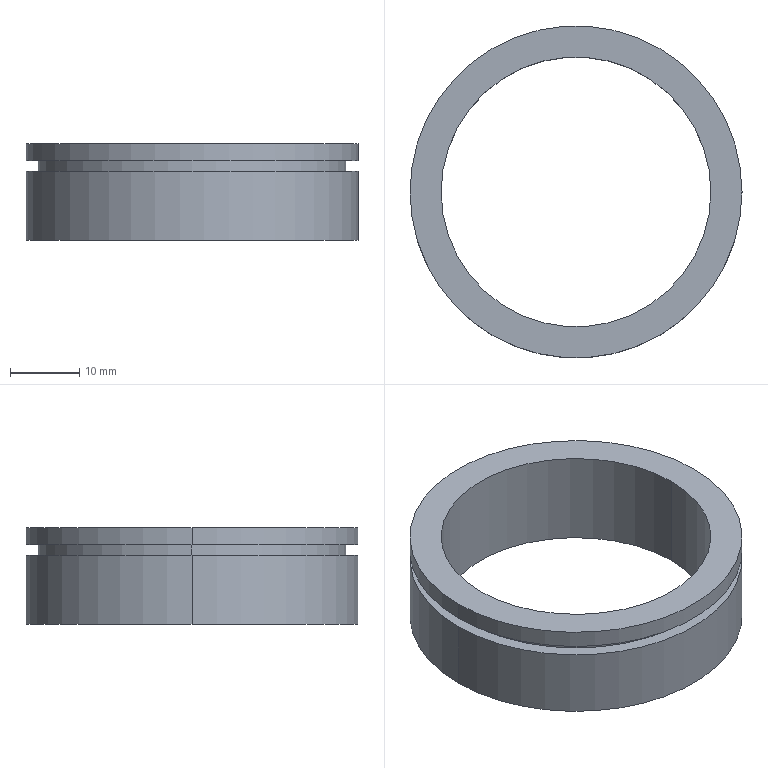Part | STEP file | Nylon bushing QY-1-28 | 1 solid | 12 faces | box 48 x 48 x 14 mm | volume 8228 mm3 | cylinder 8 | plane 4 | commonest cylinder face diameters 48 x4 39 x2 44.5 x2
STEP:
#1=CARTESIAN_POINT('',(0.,0.,0.));
#2=DIRECTION('',(0.,0.,1.));
#3=DIRECTION('',(1.,0.,0.));
#4=AXIS2_PLACEMENT_3D('',#1,#2,#3);
#5=CARTESIAN_POINT('',(22.25,0.,10.));
#6=VERTEX_POINT('',#5);
#7=CARTESIAN_POINT('',(-22.25,0.,10.));
#8=VERTEX_POINT('',#7);
#9=CARTESIAN_POINT('',(0.,0.,10.));
#10=DIRECTION('',(0.,0.,1.));
#11=DIRECTION('',(1.,0.,0.));
#12=AXIS2_PLACEMENT_3D('',#9,#10,#11);
#13=CIRCLE('',#12,22.25);
#14=CARTESIAN_POINT('',(0.,0.,10.));
#15=DIRECTION('',(0.,0.,1.));
#16=DIRECTION('',(1.,0.,0.));
#17=AXIS2_PLACEMENT_3D('',#14,#15,#16);
#18=CYLINDRICAL_SURFACE('',#17,22.25);
#19=CARTESIAN_POINT('',(0.,0.));
#20=DIRECTION('',(1.,0.));
#21=VECTOR('',#20,1.);
#22=LINE('',#19,#21);
#23=(GEOMETRIC_REPRESENTATION_CONTEXT(2)PARAMETRIC_REPRESENTATION_CONTEXT()REPRESENTATION_CONTEXT('',''));
#24=DEFINITIONAL_REPRESENTATION('',(#22),#23);
#25=PCURVE('',#18,#24);
#26=CARTESIAN_POINT('',(0.,0.,10.));
#27=DIRECTION('',(0.,0.,1.));
#28=DIRECTION('',(1.,0.,0.));
#29=AXIS2_PLACEMENT_3D('',#26,#27,#28);
#30=PLANE('',#29);
#31=CARTESIAN_POINT('',(0.,0.));
#32=DIRECTION('',(1.,0.));
#33=AXIS2_PLACEMENT_2D('',#31,#32);
#34=CIRCLE('',#33,22.25);
#35=(GEOMETRIC_REPRESENTATION_CONTEXT(2)PARAMETRIC_REPRESENTATION_CONTEXT()REPRESENTATION_CONTEXT('',''));
#36=DEFINITIONAL_REPRESENTATION('',(#34),#35);
#37=PCURVE('',#30,#36);
#38=SURFACE_CURVE('',#13,(#25,#37),.PCURVE_S1.);
#39=EDGE_CURVE('',#6,#8,#38,.T.);
#40=ORIENTED_EDGE('',*,*,#39,.T.);
#41=CARTESIAN_POINT('',(-22.25,0.,11.5));
#42=VERTEX_POINT('',#41);
#43=CARTESIAN_POINT('',(-22.25,0.,10.));
#44=DIRECTION('',(0.,0.,1.));
#45=VECTOR('',#44,1.);
#46=LINE('',#43,#45);
#47=CARTESIAN_POINT('',(3.142,0.));
#48=DIRECTION('',(0.,1.));
#49=VECTOR('',#48,1.);
#50=LINE('',#47,#49);
#51=(GEOMETRIC_REPRESENTATION_CONTEXT(2)PARAMETRIC_REPRESENTATION_CONTEXT()REPRESENTATION_CONTEXT('',''));
#52=DEFINITIONAL_REPRESENTATION('',(#50),#51);
#53=PCURVE('',#18,#52);
#54=CARTESIAN_POINT('',(0.,0.,10.));
#55=DIRECTION('',(0.,0.,1.));
#56=DIRECTION('',(1.,0.,0.));
#57=AXIS2_PLACEMENT_3D('',#54,#55,#56);
#58=CYLINDRICAL_SURFACE('',#57,22.25);
#59=CARTESIAN_POINT('',(3.142,0.));
#60=DIRECTION('',(0.,1.));
#61=VECTOR('',#60,1.);
#62=LINE('',#59,#61);
#63=(GEOMETRIC_REPRESENTATION_CONTEXT(2)PARAMETRIC_REPRESENTATION_CONTEXT()REPRESENTATION_CONTEXT('',''));
#64=DEFINITIONAL_REPRESENTATION('',(#62),#63);
#65=PCURVE('',#58,#64);
#66=SURFACE_CURVE('',#46,(#53,#65),.PCURVE_S1.);
#67=EDGE_CURVE('',#8,#42,#66,.T.);
#68=ORIENTED_EDGE('',*,*,#67,.T.);
#69=CARTESIAN_POINT('',(22.25,0.,11.5));
#70=VERTEX_POINT('',#69);
#71=CARTESIAN_POINT('',(0.,0.,11.5));
#72=DIRECTION('',(0.,0.,1.));
#73=DIRECTION('',(1.,0.,0.));
#74=AXIS2_PLACEMENT_3D('',#71,#72,#73);
#75=CIRCLE('',#74,22.25);
#76=CARTESIAN_POINT('',(0.,1.5));
#77=DIRECTION('',(1.,0.));
#78=VECTOR('',#77,1.);
#79=LINE('',#76,#78);
#80=(GEOMETRIC_REPRESENTATION_CONTEXT(2)PARAMETRIC_REPRESENTATION_CONTEXT()REPRESENTATION_CONTEXT('',''));
#81=DEFINITIONAL_REPRESENTATION('',(#79),#80);
#82=PCURVE('',#18,#81);
#83=CARTESIAN_POINT('',(0.,0.,11.5));
#84=DIRECTION('',(0.,0.,1.));
#85=DIRECTION('',(1.,0.,0.));
#86=AXIS2_PLACEMENT_3D('',#83,#84,#85);
#87=PLANE('',#86);
#88=CARTESIAN_POINT('',(0.,0.));
#89=DIRECTION('',(1.,0.));
#90=AXIS2_PLACEMENT_2D('',#88,#89);
#91=CIRCLE('',#90,22.25);
#92=(GEOMETRIC_REPRESENTATION_CONTEXT(2)PARAMETRIC_REPRESENTATION_CONTEXT()REPRESENTATION_CONTEXT('',''));
#93=DEFINITIONAL_REPRESENTATION('',(#91),#92);
#94=PCURVE('',#87,#93);
#95=SURFACE_CURVE('',#75,(#82,#94),.PCURVE_S1.);
#96=EDGE_CURVE('',#70,#42,#95,.T.);
#97=ORIENTED_EDGE('',*,*,#96,.F.);
#98=CARTESIAN_POINT('',(22.25,0.,10.));
#99=DIRECTION('',(0.,0.,1.));
#100=VECTOR('',#99,1.);
#101=LINE('',#98,#100);
#102=CARTESIAN_POINT('',(0.,0.));
#103=DIRECTION('',(0.,1.));
#104=VECTOR('',#103,1.);
#105=LINE('',#102,#104);
#106=(GEOMETRIC_REPRESENTATION_CONTEXT(2)PARAMETRIC_REPRESENTATION_CONTEXT()REPRESENTATION_CONTEXT('',''));
#107=DEFINITIONAL_REPRESENTATION('',(#105),#106);
#108=PCURVE('',#18,#107);
#109=CARTESIAN_POINT('',(6.283,0.));
#110=DIRECTION('',(0.,1.));
#111=VECTOR('',#110,1.);
#112=LINE('',#109,#111);
#113=(GEOMETRIC_REPRESENTATION_CONTEXT(2)PARAMETRIC_REPRESENTATION_CONTEXT()REPRESENTATION_CONTEXT('',''));
#114=DEFINITIONAL_REPRESENTATION('',(#112),#113);
#115=PCURVE('',#58,#114);
#116=SURFACE_CURVE('',#101,(#108,#115),.PCURVE_S1.);
#117=EDGE_CURVE('',#6,#70,#116,.T.);
#118=ORIENTED_EDGE('',*,*,#117,.F.);
#119=EDGE_LOOP('',(#40,#68,#97,#118));
#120=FACE_BOUND('',#119,.T.);
#121=ADVANCED_FACE('',(#120),#18,.T.);
#122=CARTESIAN_POINT('',(-19.5,0.,14.));
#123=VERTEX_POINT('',#122);
#124=CARTESIAN_POINT('',(-19.5,0.,0.));
#125=VERTEX_POINT('',#124);
#126=CARTESIAN_POINT('',(-19.5,0.,14.));
#127=DIRECTION('',(0.,0.,-1.));
#128=VECTOR('',#127,1.);
#129=LINE('',#126,#128);
#130=CARTESIAN_POINT('',(0.,0.,14.));
#131=DIRECTION('',(0.,0.,-1.));
#132=DIRECTION('',(-1.,0.,0.));
#133=AXIS2_PLACEMENT_3D('',#130,#131,#132);
#134=CYLINDRICAL_SURFACE('',#133,19.5);
#135=CARTESIAN_POINT('',(6.283,0.));
#136=DIRECTION('',(0.,1.));
#137=VECTOR('',#136,1.);
#138=LINE('',#135,#137);
#139=(GEOMETRIC_REPRESENTATION_CONTEXT(2)PARAMETRIC_REPRESENTATION_CONTEXT()REPRESENTATION_CONTEXT('',''));
#140=DEFINITIONAL_REPRESENTATION('',(#138),#139);
#141=PCURVE('',#134,#140);
#142=CARTESIAN_POINT('',(0.,0.,14.));
#143=DIRECTION('',(0.,0.,-1.));
#144=DIRECTION('',(-1.,0.,0.));
#145=AXIS2_PLACEMENT_3D('',#142,#143,#144);
#146=CYLINDRICAL_SURFACE('',#145,19.5);
#147=CARTESIAN_POINT('',(0.,0.));
#148=DIRECTION('',(0.,1.));
#149=VECTOR('',#148,1.);
#150=LINE('',#147,#149);
#151=(GEOMETRIC_REPRESENTATION_CONTEXT(2)PARAMETRIC_REPRESENTATION_CONTEXT()REPRESENTATION_CONTEXT('',''));
#152=DEFINITIONAL_REPRESENTATION('',(#150),#151);
#153=PCURVE('',#146,#152);
#154=SURFACE_CURVE('',#129,(#141,#153),.PCURVE_S1.);
#155=EDGE_CURVE('',#123,#125,#154,.T.);
#156=ORIENTED_EDGE('',*,*,#155,.T.);
#157=CARTESIAN_POINT('',(19.5,0.,0.));
#158=VERTEX_POINT('',#157);
#159=CARTESIAN_POINT('',(0.,0.,0.));
#160=DIRECTION('',(0.,0.,1.));
#161=DIRECTION('',(1.,0.,0.));
#162=AXIS2_PLACEMENT_3D('',#159,#160,#161);
#163=CIRCLE('',#162,19.5);
#164=CARTESIAN_POINT('',(9.425,14.));
#165=DIRECTION('',(-1.,0.));
#166=VECTOR('',#165,1.);
#167=LINE('',#164,#166);
#168=(GEOMETRIC_REPRESENTATION_CONTEXT(2)PARAMETRIC_REPRESENTATION_CONTEXT()REPRESENTATION_CONTEXT('',''));
#169=DEFINITIONAL_REPRESENTATION('',(#167),#168);
#170=PCURVE('',#134,#169);
#171=CARTESIAN_POINT('',(0.,0.,0.));
#172=DIRECTION('',(0.,0.,1.));
#173=DIRECTION('',(1.,0.,0.));
#174=AXIS2_PLACEMENT_3D('',#171,#172,#173);
#175=PLANE('',#174);
#176=CARTESIAN_POINT('',(0.,0.));
#177=DIRECTION('',(1.,0.));
#178=AXIS2_PLACEMENT_2D('',#176,#177);
#179=CIRCLE('',#178,19.5);
#180=(GEOMETRIC_REPRESENTATION_CONTEXT(2)PARAMETRIC_REPRESENTATION_CONTEXT()REPRESENTATION_CONTEXT('',''));
#181=DEFINITIONAL_REPRESENTATION('',(#179),#180);
#182=PCURVE('',#175,#181);
#183=SURFACE_CURVE('',#163,(#170,#182),.PCURVE_S1.);
#184=EDGE_CURVE('',#125,#158,#183,.T.);
#185=ORIENTED_EDGE('',*,*,#184,.T.);
#186=CARTESIAN_POINT('',(19.5,0.,14.));
#187=VERTEX_POINT('',#186);
#188=CARTESIAN_POINT('',(19.5,0.,14.));
#189=DIRECTION('',(0.,0.,-1.));
#190=VECTOR('',#189,1.);
#191=LINE('',#188,#190);
#192=CARTESIAN_POINT('',(3.142,0.));
#193=DIRECTION('',(0.,1.));
#194=VECTOR('',#193,1.);
#195=LINE('',#192,#194);
#196=(GEOMETRIC_REPRESENTATION_CONTEXT(2)PARAMETRIC_REPRESENTATION_CONTEXT()REPRESENTATION_CONTEXT('',''));
#197=DEFINITIONAL_REPRESENTATION('',(#195),#196);
#198=PCURVE('',#134,#197);
#199=CARTESIAN_POINT('',(3.142,0.));
#200=DIRECTION('',(0.,1.));
#201=VECTOR('',#200,1.);
#202=LINE('',#199,#201);
#203=(GEOMETRIC_REPRESENTATION_CONTEXT(2)PARAMETRIC_REPRESENTATION_CONTEXT()REPRESENTATION_CONTEXT('',''));
#204=DEFINITIONAL_REPRESENTATION('',(#202),#203);
#205=PCURVE('',#146,#204);
#206=SURFACE_CURVE('',#191,(#198,#205),.PCURVE_S1.);
#207=EDGE_CURVE('',#187,#158,#206,.T.);
#208=ORIENTED_EDGE('',*,*,#207,.F.);
#209=CARTESIAN_POINT('',(0.,0.,14.));
#210=DIRECTION('',(0.,0.,1.));
#211=DIRECTION('',(1.,0.,0.));
#212=AXIS2_PLACEMENT_3D('',#209,#210,#211);
#213=CIRCLE('',#212,19.5);
#214=CARTESIAN_POINT('',(9.425,0.));
#215=DIRECTION('',(-1.,0.));
#216=VECTOR('',#215,1.);
#217=LINE('',#214,#216);
#218=(GEOMETRIC_REPRESENTATION_CONTEXT(2)PARAMETRIC_REPRESENTATION_CONTEXT()REPRESENTATION_CONTEXT('',''));
#219=DEFINITIONAL_REPRESENTATION('',(#217),#218);
#220=PCURVE('',#134,#219);
#221=CARTESIAN_POINT('',(0.,0.,14.));
#222=DIRECTION('',(0.,0.,1.));
#223=DIRECTION('',(1.,0.,0.));
#224=AXIS2_PLACEMENT_3D('',#221,#222,#223);
#225=PLANE('',#224);
#226=CARTESIAN_POINT('',(0.,0.));
#227=DIRECTION('',(1.,0.));
#228=AXIS2_PLACEMENT_2D('',#226,#227);
#229=CIRCLE('',#228,19.5);
#230=(GEOMETRIC_REPRESENTATION_CONTEXT(2)PARAMETRIC_REPRESENTATION_CONTEXT()REPRESENTATION_CONTEXT('',''));
#231=DEFINITIONAL_REPRESENTATION('',(#229),#230);
#232=PCURVE('',#225,#231);
#233=SURFACE_CURVE('',#213,(#220,#232),.PCURVE_S1.);
#234=EDGE_CURVE('',#123,#187,#233,.T.);
#235=ORIENTED_EDGE('',*,*,#234,.F.);
#236=EDGE_LOOP('',(#156,#185,#208,#235));
#237=FACE_BOUND('',#236,.F.);
#238=ADVANCED_FACE('',(#237),#134,.F.);
#239=CARTESIAN_POINT('',(24.,0.,14.));
#240=VERTEX_POINT('',#239);
#241=CARTESIAN_POINT('',(-24.,0.,14.));
#242=VERTEX_POINT('',#241);
#243=CARTESIAN_POINT('',(0.,0.,14.));
#244=DIRECTION('',(0.,0.,1.));
#245=DIRECTION('',(1.,0.,0.));
#246=AXIS2_PLACEMENT_3D('',#243,#244,#245);
#247=CIRCLE('',#246,24.);
#248=CARTESIAN_POINT('',(0.,0.,14.));
#249=DIRECTION('',(0.,0.,-1.));
#250=DIRECTION('',(-1.,0.,0.));
#251=AXIS2_PLACEMENT_3D('',#248,#249,#250);
#252=CYLINDRICAL_SURFACE('',#251,24.);
#253=CARTESIAN_POINT('',(3.142,0.));
#254=DIRECTION('',(-1.,0.));
#255=VECTOR('',#254,1.);
#256=LINE('',#253,#255);
#257=(GEOMETRIC_REPRESENTATION_CONTEXT(2)PARAMETRIC_REPRESENTATION_CONTEXT()REPRESENTATION_CONTEXT('',''));
#258=DEFINITIONAL_REPRESENTATION('',(#256),#257);
#259=PCURVE('',#252,#258);
#260=CARTESIAN_POINT('',(0.,0.));
#261=DIRECTION('',(1.,0.));
#262=AXIS2_PLACEMENT_2D('',#260,#261);
#263=CIRCLE('',#262,24.);
#264=(GEOMETRIC_REPRESENTATION_CONTEXT(2)PARAMETRIC_REPRESENTATION_CONTEXT()REPRESENTATION_CONTEXT('',''));
#265=DEFINITIONAL_REPRESENTATION('',(#263),#264);
#266=PCURVE('',#225,#265);
#267=SURFACE_CURVE('',#247,(#259,#266),.PCURVE_S1.);
#268=EDGE_CURVE('',#240,#242,#267,.T.);
#269=ORIENTED_EDGE('',*,*,#268,.F.);
#270=CARTESIAN_POINT('',(24.,0.,11.5));
#271=VERTEX_POINT('',#270);
#272=CARTESIAN_POINT('',(24.,0.,14.));
#273=DIRECTION('',(0.,0.,-1.));
#274=VECTOR('',#273,1.);
#275=LINE('',#272,#274);
#276=CARTESIAN_POINT('',(3.142,0.));
#277=DIRECTION('',(0.,1.));
#278=VECTOR('',#277,1.);
#279=LINE('',#276,#278);
#280=(GEOMETRIC_REPRESENTATION_CONTEXT(2)PARAMETRIC_REPRESENTATION_CONTEXT()REPRESENTATION_CONTEXT('',''));
#281=DEFINITIONAL_REPRESENTATION('',(#279),#280);
#282=PCURVE('',#252,#281);
#283=CARTESIAN_POINT('',(0.,0.,14.));
#284=DIRECTION('',(0.,0.,-1.));
#285=DIRECTION('',(-1.,0.,0.));
#286=AXIS2_PLACEMENT_3D('',#283,#284,#285);
#287=CYLINDRICAL_SURFACE('',#286,24.);
#288=CARTESIAN_POINT('',(3.142,0.));
#289=DIRECTION('',(0.,1.));
#290=VECTOR('',#289,1.);
#291=LINE('',#288,#290);
#292=(GEOMETRIC_REPRESENTATION_CONTEXT(2)PARAMETRIC_REPRESENTATION_CONTEXT()REPRESENTATION_CONTEXT('',''));
#293=DEFINITIONAL_REPRESENTATION('',(#291),#292);
#294=PCURVE('',#287,#293);
#295=SURFACE_CURVE('',#275,(#282,#294),.PCURVE_S1.);
#296=EDGE_CURVE('',#240,#271,#295,.T.);
#297=ORIENTED_EDGE('',*,*,#296,.T.);
#298=CARTESIAN_POINT('',(-24.,0.,11.5));
#299=VERTEX_POINT('',#298);
#300=CARTESIAN_POINT('',(0.,0.,11.5));
#301=DIRECTION('',(0.,0.,1.));
#302=DIRECTION('',(1.,0.,0.));
#303=AXIS2_PLACEMENT_3D('',#300,#301,#302);
#304=CIRCLE('',#303,24.);
#305=CARTESIAN_POINT('',(3.142,2.5));
#306=DIRECTION('',(-1.,0.));
#307=VECTOR('',#306,1.);
#308=LINE('',#305,#307);
#309=(GEOMETRIC_REPRESENTATION_CONTEXT(2)PARAMETRIC_REPRESENTATION_CONTEXT()REPRESENTATION_CONTEXT('',''));
#310=DEFINITIONAL_REPRESENTATION('',(#308),#309);
#311=PCURVE('',#252,#310);
#312=CARTESIAN_POINT('',(0.,0.));
#313=DIRECTION('',(1.,0.));
#314=AXIS2_PLACEMENT_2D('',#312,#313);
#315=CIRCLE('',#314,24.);
#316=(GEOMETRIC_REPRESENTATION_CONTEXT(2)PARAMETRIC_REPRESENTATION_CONTEXT()REPRESENTATION_CONTEXT('',''));
#317=DEFINITIONAL_REPRESENTATION('',(#315),#316);
#318=PCURVE('',#87,#317);
#319=SURFACE_CURVE('',#304,(#311,#318),.PCURVE_S1.);
#320=EDGE_CURVE('',#271,#299,#319,.T.);
#321=ORIENTED_EDGE('',*,*,#320,.T.);
#322=CARTESIAN_POINT('',(-24.,0.,14.));
#323=DIRECTION('',(0.,0.,-1.));
#324=VECTOR('',#323,1.);
#325=LINE('',#322,#324);
#326=CARTESIAN_POINT('',(0.,0.));
#327=DIRECTION('',(0.,1.));
#328=VECTOR('',#327,1.);
#329=LINE('',#326,#328);
#330=(GEOMETRIC_REPRESENTATION_CONTEXT(2)PARAMETRIC_REPRESENTATION_CONTEXT()REPRESENTATION_CONTEXT('',''));
#331=DEFINITIONAL_REPRESENTATION('',(#329),#330);
#332=PCURVE('',#252,#331);
#333=CARTESIAN_POINT('',(6.283,0.));
#334=DIRECTION('',(0.,1.));
#335=VECTOR('',#334,1.);
#336=LINE('',#333,#335);
#337=(GEOMETRIC_REPRESENTATION_CONTEXT(2)PARAMETRIC_REPRESENTATION_CONTEXT()REPRESENTATION_CONTEXT('',''));
#338=DEFINITIONAL_REPRESENTATION('',(#336),#337);
#339=PCURVE('',#287,#338);
#340=SURFACE_CURVE('',#325,(#332,#339),.PCURVE_S1.);
#341=EDGE_CURVE('',#242,#299,#340,.T.);
#342=ORIENTED_EDGE('',*,*,#341,.F.);
#343=EDGE_LOOP('',(#269,#297,#321,#342));
#344=FACE_BOUND('',#343,.T.);
#345=ADVANCED_FACE('',(#344),#252,.T.);
#346=CARTESIAN_POINT('',(24.,0.,10.));
#347=VERTEX_POINT('',#346);
#348=CARTESIAN_POINT('',(-24.,0.,10.));
#349=VERTEX_POINT('',#348);
#350=CARTESIAN_POINT('',(0.,0.,10.));
#351=DIRECTION('',(0.,0.,1.));
#352=DIRECTION('',(1.,0.,0.));
#353=AXIS2_PLACEMENT_3D('',#350,#351,#352);
#354=CIRCLE('',#353,24.);
#355=CARTESIAN_POINT('',(0.,0.,14.));
#356=DIRECTION('',(0.,0.,-1.));
#357=DIRECTION('',(-1.,0.,0.));
#358=AXIS2_PLACEMENT_3D('',#355,#356,#357);
#359=CYLINDRICAL_SURFACE('',#358,24.);
#360=CARTESIAN_POINT('',(3.142,4.));
#361=DIRECTION('',(-1.,0.));
#362=VECTOR('',#361,1.);
#363=LINE('',#360,#362);
#364=(GEOMETRIC_REPRESENTATION_CONTEXT(2)PARAMETRIC_REPRESENTATION_CONTEXT()REPRESENTATION_CONTEXT('',''));
#365=DEFINITIONAL_REPRESENTATION('',(#363),#364);
#366=PCURVE('',#359,#365);
#367=CARTESIAN_POINT('',(0.,0.));
#368=DIRECTION('',(1.,0.));
#369=AXIS2_PLACEMENT_2D('',#367,#368);
#370=CIRCLE('',#369,24.);
#371=(GEOMETRIC_REPRESENTATION_CONTEXT(2)PARAMETRIC_REPRESENTATION_CONTEXT()REPRESENTATION_CONTEXT('',''));
#372=DEFINITIONAL_REPRESENTATION('',(#370),#371);
#373=PCURVE('',#30,#372);
#374=SURFACE_CURVE('',#354,(#366,#373),.PCURVE_S1.);
#375=EDGE_CURVE('',#347,#349,#374,.T.);
#376=ORIENTED_EDGE('',*,*,#375,.F.);
#377=CARTESIAN_POINT('',(24.,0.,0.));
#378=VERTEX_POINT('',#377);
#379=CARTESIAN_POINT('',(24.,0.,14.));
#380=DIRECTION('',(0.,0.,-1.));
#381=VECTOR('',#380,1.);
#382=LINE('',#379,#381);
#383=CARTESIAN_POINT('',(3.142,0.));
#384=DIRECTION('',(0.,1.));
#385=VECTOR('',#384,1.);
#386=LINE('',#383,#385);
#387=(GEOMETRIC_REPRESENTATION_CONTEXT(2)PARAMETRIC_REPRESENTATION_CONTEXT()REPRESENTATION_CONTEXT('',''));
#388=DEFINITIONAL_REPRESENTATION('',(#386),#387);
#389=PCURVE('',#359,#388);
#390=CARTESIAN_POINT('',(0.,0.,14.));
#391=DIRECTION('',(0.,0.,-1.));
#392=DIRECTION('',(-1.,0.,0.));
#393=AXIS2_PLACEMENT_3D('',#390,#391,#392);
#394=CYLINDRICAL_SURFACE('',#393,24.);
#395=CARTESIAN_POINT('',(3.142,0.));
#396=DIRECTION('',(0.,1.));
#397=VECTOR('',#396,1.);
#398=LINE('',#395,#397);
#399=(GEOMETRIC_REPRESENTATION_CONTEXT(2)PARAMETRIC_REPRESENTATION_CONTEXT()REPRESENTATION_CONTEXT('',''));
#400=DEFINITIONAL_REPRESENTATION('',(#398),#399);
#401=PCURVE('',#394,#400);
#402=SURFACE_CURVE('',#382,(#389,#401),.PCURVE_S1.);
#403=EDGE_CURVE('',#347,#378,#402,.T.);
#404=ORIENTED_EDGE('',*,*,#403,.T.);
#405=CARTESIAN_POINT('',(-24.,0.,0.));
#406=VERTEX_POINT('',#405);
#407=CARTESIAN_POINT('',(0.,0.,0.));
#408=DIRECTION('',(0.,0.,1.));
#409=DIRECTION('',(1.,0.,0.));
#410=AXIS2_PLACEMENT_3D('',#407,#408,#409);
#411=CIRCLE('',#410,24.);
#412=CARTESIAN_POINT('',(3.142,14.));
#413=DIRECTION('',(-1.,0.));
#414=VECTOR('',#413,1.);
#415=LINE('',#412,#414);
#416=(GEOMETRIC_REPRESENTATION_CONTEXT(2)PARAMETRIC_REPRESENTATION_CONTEXT()REPRESENTATION_CONTEXT('',''));
#417=DEFINITIONAL_REPRESENTATION('',(#415),#416);
#418=PCURVE('',#359,#417);
#419=CARTESIAN_POINT('',(0.,0.));
#420=DIRECTION('',(1.,0.));
#421=AXIS2_PLACEMENT_2D('',#419,#420);
#422=CIRCLE('',#421,24.);
#423=(GEOMETRIC_REPRESENTATION_CONTEXT(2)PARAMETRIC_REPRESENTATION_CONTEXT()REPRESENTATION_CONTEXT('',''));
#424=DEFINITIONAL_REPRESENTATION('',(#422),#423);
#425=PCURVE('',#175,#424);
#426=SURFACE_CURVE('',#411,(#418,#425),.PCURVE_S1.);
#427=EDGE_CURVE('',#378,#406,#426,.T.);
#428=ORIENTED_EDGE('',*,*,#427,.T.);
#429=CARTESIAN_POINT('',(-24.,0.,14.));
#430=DIRECTION('',(0.,0.,-1.));
#431=VECTOR('',#430,1.);
#432=LINE('',#429,#431);
#433=CARTESIAN_POINT('',(0.,0.));
#434=DIRECTION('',(0.,1.));
#435=VECTOR('',#434,1.);
#436=LINE('',#433,#435);
#437=(GEOMETRIC_REPRESENTATION_CONTEXT(2)PARAMETRIC_REPRESENTATION_CONTEXT()REPRESENTATION_CONTEXT('',''));
#438=DEFINITIONAL_REPRESENTATION('',(#436),#437);
#439=PCURVE('',#359,#438);
#440=CARTESIAN_POINT('',(6.283,0.));
#441=DIRECTION('',(0.,1.));
#442=VECTOR('',#441,1.);
#443=LINE('',#440,#442);
#444=(GEOMETRIC_REPRESENTATION_CONTEXT(2)PARAMETRIC_REPRESENTATION_CONTEXT()REPRESENTATION_CONTEXT('',''));
#445=DEFINITIONAL_REPRESENTATION('',(#443),#444);
#446=PCURVE('',#394,#445);
#447=SURFACE_CURVE('',#432,(#439,#446),.PCURVE_S1.);
#448=EDGE_CURVE('',#349,#406,#447,.T.);
#449=ORIENTED_EDGE('',*,*,#448,.F.);
#450=EDGE_LOOP('',(#376,#404,#428,#449));
#451=FACE_BOUND('',#450,.T.);
#452=ADVANCED_FACE('',(#451),#359,.T.);
#453=ORIENTED_EDGE('',*,*,#403,.F.);
#454=CARTESIAN_POINT('',(0.,0.,10.));
#455=DIRECTION('',(0.,0.,1.));
#456=DIRECTION('',(1.,0.,0.));
#457=AXIS2_PLACEMENT_3D('',#454,#455,#456);
#458=CIRCLE('',#457,24.);
#459=CARTESIAN_POINT('',(9.425,4.));
#460=DIRECTION('',(-1.,0.));
#461=VECTOR('',#460,1.);
#462=LINE('',#459,#461);
#463=(GEOMETRIC_REPRESENTATION_CONTEXT(2)PARAMETRIC_REPRESENTATION_CONTEXT()REPRESENTATION_CONTEXT('',''));
#464=DEFINITIONAL_REPRESENTATION('',(#462),#463);
#465=PCURVE('',#394,#464);
#466=CARTESIAN_POINT('',(0.,0.));
#467=DIRECTION('',(1.,0.));
#468=AXIS2_PLACEMENT_2D('',#466,#467);
#469=CIRCLE('',#468,24.);
#470=(GEOMETRIC_REPRESENTATION_CONTEXT(2)PARAMETRIC_REPRESENTATION_CONTEXT()REPRESENTATION_CONTEXT('',''));
#471=DEFINITIONAL_REPRESENTATION('',(#469),#470);
#472=PCURVE('',#30,#471);
#473=SURFACE_CURVE('',#458,(#465,#472),.PCURVE_S1.);
#474=EDGE_CURVE('',#349,#347,#473,.T.);
#475=ORIENTED_EDGE('',*,*,#474,.F.);
#476=ORIENTED_EDGE('',*,*,#448,.T.);
#477=CARTESIAN_POINT('',(0.,0.,0.));
#478=DIRECTION('',(0.,0.,1.));
#479=DIRECTION('',(1.,0.,0.));
#480=AXIS2_PLACEMENT_3D('',#477,#478,#479);
#481=CIRCLE('',#480,24.);
#482=CARTESIAN_POINT('',(9.425,14.));
#483=DIRECTION('',(-1.,0.));
#484=VECTOR('',#483,1.);
#485=LINE('',#482,#484);
#486=(GEOMETRIC_REPRESENTATION_CONTEXT(2)PARAMETRIC_REPRESENTATION_CONTEXT()REPRESENTATION_CONTEXT('',''));
#487=DEFINITIONAL_REPRESENTATION('',(#485),#486);
#488=PCURVE('',#394,#487);
#489=CARTESIAN_POINT('',(0.,0.));
#490=DIRECTION('',(1.,0.));
#491=AXIS2_PLACEMENT_2D('',#489,#490);
#492=CIRCLE('',#491,24.);
#493=(GEOMETRIC_REPRESENTATION_CONTEXT(2)PARAMETRIC_REPRESENTATION_CONTEXT()REPRESENTATION_CONTEXT('',''));
#494=DEFINITIONAL_REPRESENTATION('',(#492),#493);
#495=PCURVE('',#175,#494);
#496=SURFACE_CURVE('',#481,(#488,#495),.PCURVE_S1.);
#497=EDGE_CURVE('',#406,#378,#496,.T.);
#498=ORIENTED_EDGE('',*,*,#497,.T.);
#499=EDGE_LOOP('',(#453,#475,#476,#498));
#500=FACE_BOUND('',#499,.T.);
#501=ADVANCED_FACE('',(#500),#394,.T.);
#502=CARTESIAN_POINT('',(0.,0.,14.));
#503=DIRECTION('',(0.,0.,1.));
#504=DIRECTION('',(1.,0.,0.));
#505=AXIS2_PLACEMENT_3D('',#502,#503,#504);
#506=CIRCLE('',#505,24.);
#507=CARTESIAN_POINT('',(0.,0.));
#508=DIRECTION('',(1.,0.));
#509=AXIS2_PLACEMENT_2D('',#507,#508);
#510=CIRCLE('',#509,24.);
#511=(GEOMETRIC_REPRESENTATION_CONTEXT(2)PARAMETRIC_REPRESENTATION_CONTEXT()REPRESENTATION_CONTEXT('',''));
#512=DEFINITIONAL_REPRESENTATION('',(#510),#511);
#513=PCURVE('',#225,#512);
#514=CARTESIAN_POINT('',(9.425,0.));
#515=DIRECTION('',(-1.,0.));
#516=VECTOR('',#515,1.);
#517=LINE('',#514,#516);
#518=(GEOMETRIC_REPRESENTATION_CONTEXT(2)PARAMETRIC_REPRESENTATION_CONTEXT()REPRESENTATION_CONTEXT('',''));
#519=DEFINITIONAL_REPRESENTATION('',(#517),#518);
#520=PCURVE('',#287,#519);
#521=SURFACE_CURVE('',#506,(#513,#520),.PCURVE_S1.);
#522=EDGE_CURVE('',#242,#240,#521,.T.);
#523=ORIENTED_EDGE('',*,*,#522,.T.);
#524=ORIENTED_EDGE('',*,*,#268,.T.);
#525=EDGE_LOOP('',(#523,#524));
#526=FACE_BOUND('',#525,.T.);
#527=ORIENTED_EDGE('',*,*,#234,.F.);
#528=CARTESIAN_POINT('',(0.,0.,14.));
#529=DIRECTION('',(0.,0.,1.));
#530=DIRECTION('',(1.,0.,0.));
#531=AXIS2_PLACEMENT_3D('',#528,#529,#530);
#532=CIRCLE('',#531,19.5);
#533=CARTESIAN_POINT('',(0.,0.));
#534=DIRECTION('',(1.,0.));
#535=AXIS2_PLACEMENT_2D('',#533,#534);
#536=CIRCLE('',#535,19.5);
#537=(GEOMETRIC_REPRESENTATION_CONTEXT(2)PARAMETRIC_REPRESENTATION_CONTEXT()REPRESENTATION_CONTEXT('',''));
#538=DEFINITIONAL_REPRESENTATION('',(#536),#537);
#539=PCURVE('',#225,#538);
#540=CARTESIAN_POINT('',(3.142,0.));
#541=DIRECTION('',(-1.,0.));
#542=VECTOR('',#541,1.);
#543=LINE('',#540,#542);
#544=(GEOMETRIC_REPRESENTATION_CONTEXT(2)PARAMETRIC_REPRESENTATION_CONTEXT()REPRESENTATION_CONTEXT('',''));
#545=DEFINITIONAL_REPRESENTATION('',(#543),#544);
#546=PCURVE('',#146,#545);
#547=SURFACE_CURVE('',#532,(#539,#546),.PCURVE_S1.);
#548=EDGE_CURVE('',#187,#123,#547,.T.);
#549=ORIENTED_EDGE('',*,*,#548,.F.);
#550=EDGE_LOOP('',(#527,#549));
#551=FACE_BOUND('',#550,.T.);
#552=ADVANCED_FACE('',(#526,#551),#225,.T.);
#553=ORIENTED_EDGE('',*,*,#497,.F.);
#554=ORIENTED_EDGE('',*,*,#427,.F.);
#555=EDGE_LOOP('',(#553,#554));
#556=FACE_BOUND('',#555,.T.);
#557=ORIENTED_EDGE('',*,*,#184,.T.);
#558=CARTESIAN_POINT('',(0.,0.,0.));
#559=DIRECTION('',(0.,0.,1.));
#560=DIRECTION('',(1.,0.,0.));
#561=AXIS2_PLACEMENT_3D('',#558,#559,#560);
#562=CIRCLE('',#561,19.5);
#563=CARTESIAN_POINT('',(0.,0.));
#564=DIRECTION('',(1.,0.));
#565=AXIS2_PLACEMENT_2D('',#563,#564);
#566=CIRCLE('',#565,19.5);
#567=(GEOMETRIC_REPRESENTATION_CONTEXT(2)PARAMETRIC_REPRESENTATION_CONTEXT()REPRESENTATION_CONTEXT('',''));
#568=DEFINITIONAL_REPRESENTATION('',(#566),#567);
#569=PCURVE('',#175,#568);
#570=CARTESIAN_POINT('',(3.142,14.));
#571=DIRECTION('',(-1.,0.));
#572=VECTOR('',#571,1.);
#573=LINE('',#570,#572);
#574=(GEOMETRIC_REPRESENTATION_CONTEXT(2)PARAMETRIC_REPRESENTATION_CONTEXT()REPRESENTATION_CONTEXT('',''));
#575=DEFINITIONAL_REPRESENTATION('',(#573),#574);
#576=PCURVE('',#146,#575);
#577=SURFACE_CURVE('',#562,(#569,#576),.PCURVE_S1.);
#578=EDGE_CURVE('',#158,#125,#577,.T.);
#579=ORIENTED_EDGE('',*,*,#578,.T.);
#580=EDGE_LOOP('',(#557,#579));
#581=FACE_BOUND('',#580,.T.);
#582=ADVANCED_FACE('',(#556,#581),#175,.F.);
#583=ORIENTED_EDGE('',*,*,#296,.F.);
#584=ORIENTED_EDGE('',*,*,#522,.F.);
#585=ORIENTED_EDGE('',*,*,#341,.T.);
#586=CARTESIAN_POINT('',(0.,0.,11.5));
#587=DIRECTION('',(0.,0.,1.));
#588=DIRECTION('',(1.,0.,0.));
#589=AXIS2_PLACEMENT_3D('',#586,#587,#588);
#590=CIRCLE('',#589,24.);
#591=CARTESIAN_POINT('',(9.425,2.5));
#592=DIRECTION('',(-1.,0.));
#593=VECTOR('',#592,1.);
#594=LINE('',#591,#593);
#595=(GEOMETRIC_REPRESENTATION_CONTEXT(2)PARAMETRIC_REPRESENTATION_CONTEXT()REPRESENTATION_CONTEXT('',''));
#596=DEFINITIONAL_REPRESENTATION('',(#594),#595);
#597=PCURVE('',#287,#596);
#598=CARTESIAN_POINT('',(0.,0.));
#599=DIRECTION('',(1.,0.));
#600=AXIS2_PLACEMENT_2D('',#598,#599);
#601=CIRCLE('',#600,24.);
#602=(GEOMETRIC_REPRESENTATION_CONTEXT(2)PARAMETRIC_REPRESENTATION_CONTEXT()REPRESENTATION_CONTEXT('',''));
#603=DEFINITIONAL_REPRESENTATION('',(#601),#602);
#604=PCURVE('',#87,#603);
#605=SURFACE_CURVE('',#590,(#597,#604),.PCURVE_S1.);
#606=EDGE_CURVE('',#299,#271,#605,.T.);
#607=ORIENTED_EDGE('',*,*,#606,.T.);
#608=EDGE_LOOP('',(#583,#584,#585,#607));
#609=FACE_BOUND('',#608,.T.);
#610=ADVANCED_FACE('',(#609),#287,.T.);
#611=ORIENTED_EDGE('',*,*,#578,.T.);
#612=ORIENTED_EDGE('',*,*,#155,.F.);
#613=ORIENTED_EDGE('',*,*,#548,.F.);
#614=ORIENTED_EDGE('',*,*,#207,.T.);
#615=EDGE_LOOP('',(#611,#612,#613,#614));
#616=FACE_BOUND('',#615,.F.);
#617=ADVANCED_FACE('',(#616),#146,.F.);
#618=ORIENTED_EDGE('',*,*,#39,.F.);
#619=CARTESIAN_POINT('',(0.,0.,10.));
#620=DIRECTION('',(0.,0.,1.));
#621=DIRECTION('',(1.,0.,0.));
#622=AXIS2_PLACEMENT_3D('',#619,#620,#621);
#623=CIRCLE('',#622,22.25);
#624=CARTESIAN_POINT('',(0.,0.));
#625=DIRECTION('',(1.,0.));
#626=AXIS2_PLACEMENT_2D('',#624,#625);
#627=CIRCLE('',#626,22.25);
#628=(GEOMETRIC_REPRESENTATION_CONTEXT(2)PARAMETRIC_REPRESENTATION_CONTEXT()REPRESENTATION_CONTEXT('',''));
#629=DEFINITIONAL_REPRESENTATION('',(#627),#628);
#630=PCURVE('',#30,#629);
#631=CARTESIAN_POINT('',(0.,0.));
#632=DIRECTION('',(1.,0.));
#633=VECTOR('',#632,1.);
#634=LINE('',#631,#633);
#635=(GEOMETRIC_REPRESENTATION_CONTEXT(2)PARAMETRIC_REPRESENTATION_CONTEXT()REPRESENTATION_CONTEXT('',''));
#636=DEFINITIONAL_REPRESENTATION('',(#634),#635);
#637=PCURVE('',#58,#636);
#638=SURFACE_CURVE('',#623,(#630,#637),.PCURVE_S1.);
#639=EDGE_CURVE('',#8,#6,#638,.T.);
#640=ORIENTED_EDGE('',*,*,#639,.F.);
#641=EDGE_LOOP('',(#618,#640));
#642=FACE_BOUND('',#641,.T.);
#643=ORIENTED_EDGE('',*,*,#474,.T.);
#644=ORIENTED_EDGE('',*,*,#375,.T.);
#645=EDGE_LOOP('',(#643,#644));
#646=FACE_BOUND('',#645,.T.);
#647=ADVANCED_FACE('',(#642,#646),#30,.T.);
#648=ORIENTED_EDGE('',*,*,#96,.T.);
#649=CARTESIAN_POINT('',(0.,0.,11.5));
#650=DIRECTION('',(0.,0.,1.));
#651=DIRECTION('',(1.,0.,0.));
#652=AXIS2_PLACEMENT_3D('',#649,#650,#651);
#653=CIRCLE('',#652,22.25);
#654=CARTESIAN_POINT('',(0.,0.));
#655=DIRECTION('',(1.,0.));
#656=AXIS2_PLACEMENT_2D('',#654,#655);
#657=CIRCLE('',#656,22.25);
#658=(GEOMETRIC_REPRESENTATION_CONTEXT(2)PARAMETRIC_REPRESENTATION_CONTEXT()REPRESENTATION_CONTEXT('',''));
#659=DEFINITIONAL_REPRESENTATION('',(#657),#658);
#660=PCURVE('',#87,#659);
#661=CARTESIAN_POINT('',(0.,1.5));
#662=DIRECTION('',(1.,0.));
#663=VECTOR('',#662,1.);
#664=LINE('',#661,#663);
#665=(GEOMETRIC_REPRESENTATION_CONTEXT(2)PARAMETRIC_REPRESENTATION_CONTEXT()REPRESENTATION_CONTEXT('',''));
#666=DEFINITIONAL_REPRESENTATION('',(#664),#665);
#667=PCURVE('',#58,#666);
#668=SURFACE_CURVE('',#653,(#660,#667),.PCURVE_S1.);
#669=EDGE_CURVE('',#42,#70,#668,.T.);
#670=ORIENTED_EDGE('',*,*,#669,.T.);
#671=EDGE_LOOP('',(#648,#670));
#672=FACE_BOUND('',#671,.T.);
#673=ORIENTED_EDGE('',*,*,#606,.F.);
#674=ORIENTED_EDGE('',*,*,#320,.F.);
#675=EDGE_LOOP('',(#673,#674));
#676=FACE_BOUND('',#675,.T.);
#677=ADVANCED_FACE('',(#672,#676),#87,.F.);
#678=ORIENTED_EDGE('',*,*,#67,.F.);
#679=ORIENTED_EDGE('',*,*,#639,.T.);
#680=ORIENTED_EDGE('',*,*,#117,.T.);
#681=ORIENTED_EDGE('',*,*,#669,.F.);
#682=EDGE_LOOP('',(#678,#679,#680,#681));
#683=FACE_BOUND('',#682,.T.);
#684=ADVANCED_FACE('',(#683),#58,.T.);
#685=CLOSED_SHELL('',(#121,#238,#345,#452,#501,#552,#582,#610,#617,#647,#677,#684));
#686=MANIFOLD_SOLID_BREP('',#685);
#687=(LENGTH_UNIT()NAMED_UNIT(*)SI_UNIT(.MILLI.,.METRE.));
#688=UNCERTAINTY_MEASURE_WITH_UNIT(LENGTH_MEASURE(0.0000001),#687,'','');
#689=(NAMED_UNIT(*)PLANE_ANGLE_UNIT()SI_UNIT($,.RADIAN.));
#690=(NAMED_UNIT(*)SI_UNIT($,.STERADIAN.)SOLID_ANGLE_UNIT());
#691=(GEOMETRIC_REPRESENTATION_CONTEXT(3)GLOBAL_UNCERTAINTY_ASSIGNED_CONTEXT((#688))GLOBAL_UNIT_ASSIGNED_CONTEXT((#687,#689,#690))REPRESENTATION_CONTEXT('',''));
#692=ADVANCED_BREP_SHAPE_REPRESENTATION('',(#4,#686),#691);